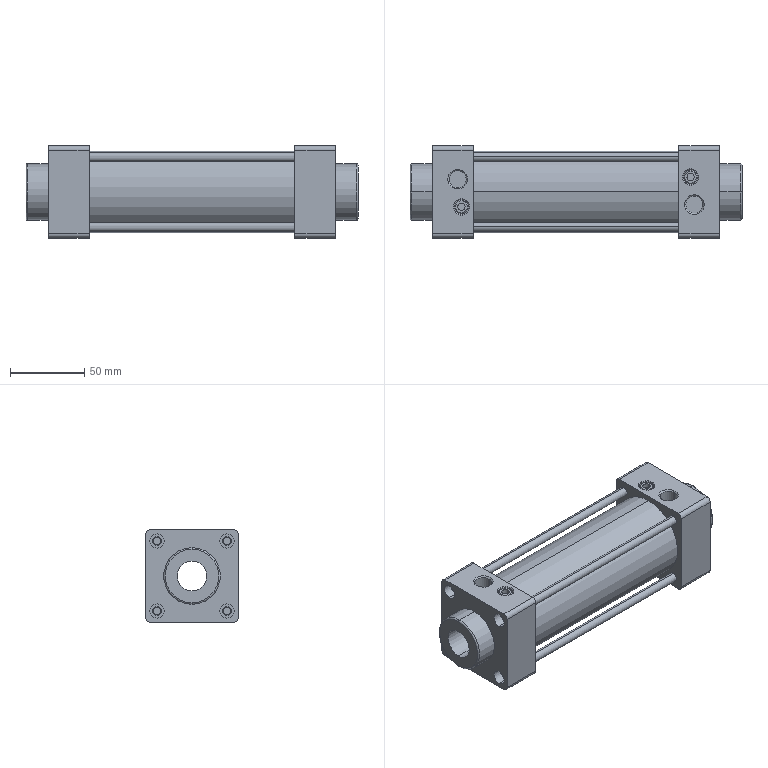Part | SolidWorks | features RefAxis 48, 3DProfileFeature 16, RevCut 7, LPattern 3, Revolution 3, ICE 2, Extrusion 1 | 1 solid | 154 faces | box 223 x 62 x 62 mm | volume 281085 mm3 | cylinder 80 | plane 42 | cone 28 | torus 4 | commonest cylinder face diameters 4.917 x16 6 x16 9.5 x16 5 x4 9.1 x4 10.1 x4